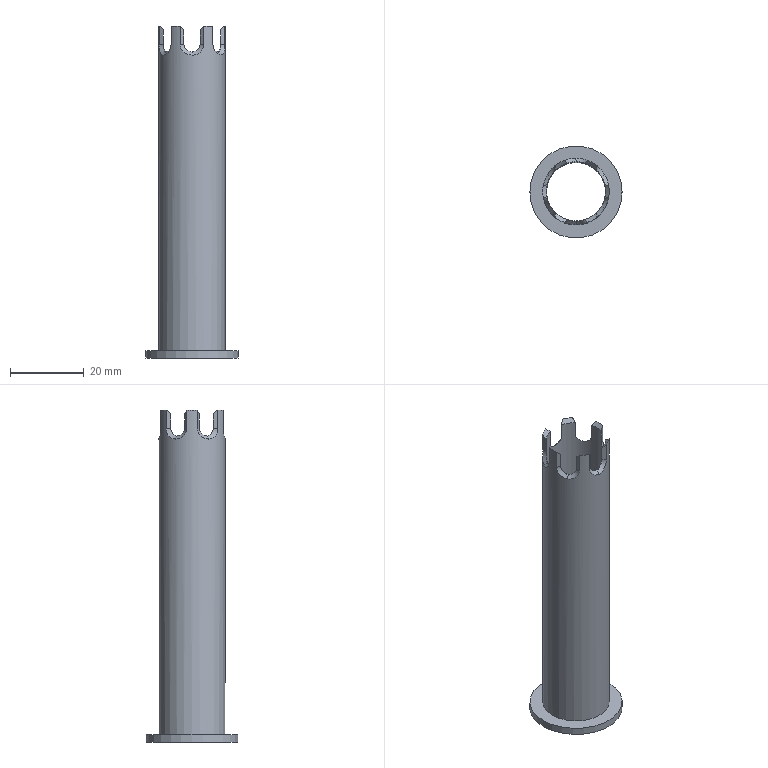Part | NX | features DATUM_CSYS 5, SKETCH 4, EXTRUDE 3, BLEND 2, CHAMFER 2 | 1 solid | 47 faces | box 25 x 25 x 90 mm | volume 5042 mm3 | cylinder 15 | plane 14 | spline 12 | cone 6 | commonest cylinder face diameters 4 x12 16 x1 18 x1 25 x1